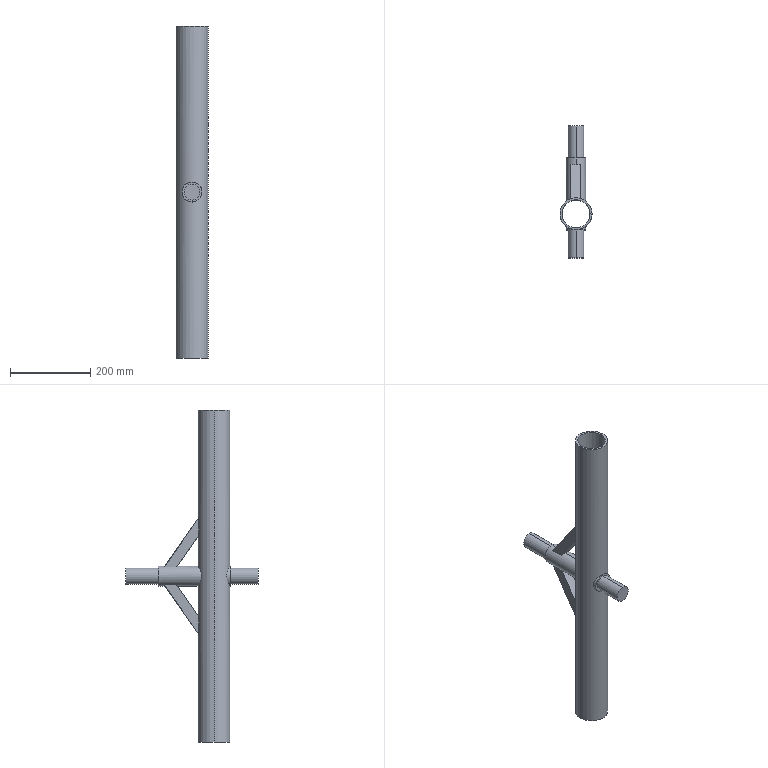Part | SolidWorks | 1 solid | 26 faces | box 80 x 330 x 830 mm | volume 1520421 mm3 | plane 14 | cylinder 12 | commonest cylinder face diameters 40 x4 50 x4 70 x2 80 x2
STEP:
#1=CARTESIAN_POINT('',(0.,140.,20.));
#2=VERTEX_POINT('',#1);
#3=CARTESIAN_POINT('',(0.,140.,-20.));
#4=VERTEX_POINT('',#3);
#5=CARTESIAN_POINT('',(0.,140.,0.));
#6=DIRECTION('',(0.,1.,0.));
#7=DIRECTION('',(0.,0.,1.));
#8=AXIS2_PLACEMENT_3D('',#5,#6,#7);
#9=CIRCLE('',#8,20.);
#10=EDGE_CURVE('',#2,#4,#9,.T.);
#11=ORIENTED_EDGE('',*,*,#10,.T.);
#12=CARTESIAN_POINT('',(0.,220.,-20.));
#13=VERTEX_POINT('',#12);
#14=CARTESIAN_POINT('',(0.,-236.569,-20.));
#15=DIRECTION('',(0.,1.,0.));
#16=VECTOR('',#15,1000.);
#17=LINE('',#14,#16);
#18=EDGE_CURVE('',#4,#13,#17,.T.);
#19=ORIENTED_EDGE('',*,*,#18,.T.);
#20=CARTESIAN_POINT('',(0.,220.,20.));
#21=VERTEX_POINT('',#20);
#22=CARTESIAN_POINT('',(0.,220.,0.));
#23=DIRECTION('',(0.,1.,0.));
#24=DIRECTION('',(0.,0.,1.));
#25=AXIS2_PLACEMENT_3D('',#22,#23,#24);
#26=CIRCLE('',#25,20.);
#27=EDGE_CURVE('',#21,#13,#26,.T.);
#28=ORIENTED_EDGE('',*,*,#27,.F.);
#29=CARTESIAN_POINT('',(0.,-236.569,20.));
#30=DIRECTION('',(0.,1.,0.));
#31=VECTOR('',#30,1000.);
#32=LINE('',#29,#31);
#33=EDGE_CURVE('',#2,#21,#32,.T.);
#34=ORIENTED_EDGE('',*,*,#33,.F.);
#35=EDGE_LOOP('',(#11,#19,#28,#34));
#36=FACE_OUTER_BOUND('',#35,.T.);
#37=CARTESIAN_POINT('',(0.,-236.569,0.));
#38=DIRECTION('',(0.,1.,0.));
#39=DIRECTION('',(0.,0.,1.));
#40=AXIS2_PLACEMENT_3D('',#37,#38,#39);
#41=CYLINDRICAL_SURFACE('',#40,20.);
#42=ADVANCED_FACE('',(#36),#41,.T.);
#43=CARTESIAN_POINT('',(0.,-110.,-20.));
#44=VERTEX_POINT('',#43);
#45=CARTESIAN_POINT('',(0.,-110.,20.));
#46=VERTEX_POINT('',#45);
#47=CARTESIAN_POINT('',(0.,-110.,0.));
#48=DIRECTION('',(0.,-1.,0.));
#49=DIRECTION('',(0.,0.,1.));
#50=AXIS2_PLACEMENT_3D('',#47,#48,#49);
#51=CIRCLE('',#50,20.);
#52=EDGE_CURVE('',#44,#46,#51,.T.);
#53=ORIENTED_EDGE('',*,*,#52,.F.);
#54=CARTESIAN_POINT('',(0.,-40.,-20.));
#55=VERTEX_POINT('',#54);
#56=CARTESIAN_POINT('',(0.,-236.569,-20.));
#57=DIRECTION('',(0.,1.,0.));
#58=VECTOR('',#57,1000.);
#59=LINE('',#56,#58);
#60=EDGE_CURVE('',#44,#55,#59,.T.);
#61=ORIENTED_EDGE('',*,*,#60,.T.);
#62=CARTESIAN_POINT('',(0.,-40.,20.));
#63=VERTEX_POINT('',#62);
#64=CARTESIAN_POINT('',(0.,-40.,0.));
#65=DIRECTION('',(0.,1.,0.));
#66=DIRECTION('',(0.,0.,1.));
#67=AXIS2_PLACEMENT_3D('',#64,#65,#66);
#68=CIRCLE('',#67,20.);
#69=EDGE_CURVE('',#63,#55,#68,.T.);
#70=ORIENTED_EDGE('',*,*,#69,.F.);
#71=CARTESIAN_POINT('',(0.,-236.569,20.));
#72=DIRECTION('',(0.,1.,0.));
#73=VECTOR('',#72,1000.);
#74=LINE('',#71,#73);
#75=EDGE_CURVE('',#46,#63,#74,.T.);
#76=ORIENTED_EDGE('',*,*,#75,.F.);
#77=EDGE_LOOP('',(#53,#61,#70,#76));
#78=FACE_OUTER_BOUND('',#77,.T.);
#79=CARTESIAN_POINT('',(0.,-236.569,0.));
#80=DIRECTION('',(0.,1.,0.));
#81=DIRECTION('',(0.,0.,1.));
#82=AXIS2_PLACEMENT_3D('',#79,#80,#81);
#83=CYLINDRICAL_SURFACE('',#82,20.);
#84=ADVANCED_FACE('',(#78),#83,.T.);
#85=CARTESIAN_POINT('',(0.,40.,-25.));
#86=VERTEX_POINT('',#85);
#87=CARTESIAN_POINT('',(0.,40.,25.));
#88=VERTEX_POINT('',#87);
#89=CARTESIAN_POINT('',(0.,40.,-25.));
#90=CARTESIAN_POINT('',(1.686,40.,-25.));
#91=CARTESIAN_POINT('',(3.35,39.894,-24.831));
#92=CARTESIAN_POINT('',(5.812,39.584,-24.329));
#93=CARTESIAN_POINT('',(6.63,39.455,-24.119));
#94=CARTESIAN_POINT('',(8.216,39.155,-23.626));
#95=CARTESIAN_POINT('',(8.989,38.985,-23.342));
#96=CARTESIAN_POINT('',(10.497,38.606,-22.704));
#97=CARTESIAN_POINT('',(11.232,38.398,-22.35));
#98=CARTESIAN_POINT('',(12.307,38.062,-21.765));
#99=CARTESIAN_POINT('',(12.661,37.945,-21.561));
#100=CARTESIAN_POINT('',(13.355,37.706,-21.138));
#101=CARTESIAN_POINT('',(13.695,37.584,-20.919));
#102=CARTESIAN_POINT('',(15.361,36.96,-19.789));
#103=CARTESIAN_POINT('',(16.586,36.421,-18.773));
#104=CARTESIAN_POINT('',(18.275,35.587,-17.078));
#105=CARTESIAN_POINT('',(18.814,35.304,-16.483));
#106=CARTESIAN_POINT('',(19.824,34.747,-15.253));
#107=CARTESIAN_POINT('',(20.297,34.472,-14.617));
#108=CARTESIAN_POINT('',(21.626,33.666,-12.642));
#109=CARTESIAN_POINT('',(22.391,33.155,-11.239));
#110=CARTESIAN_POINT('',(23.348,32.481,-8.975));
#111=CARTESIAN_POINT('',(23.63,32.276,-8.204));
#112=CARTESIAN_POINT('',(24.117,31.913,-6.636));
#113=CARTESIAN_POINT('',(24.323,31.756,-5.838));
#114=CARTESIAN_POINT('',(24.574,31.562,-4.617));
#115=CARTESIAN_POINT('',(24.647,31.504,-4.206));
#116=CARTESIAN_POINT('',(24.775,31.404,-3.376));
#117=CARTESIAN_POINT('',(24.828,31.362,-2.956));
#118=CARTESIAN_POINT('',(24.957,31.26,-1.692));
#119=CARTESIAN_POINT('',(25.,31.225,-0.8513));
#120=CARTESIAN_POINT('',(25.,31.225,0.8251));
#121=CARTESIAN_POINT('',(24.959,31.258,1.661));
#122=CARTESIAN_POINT('',(24.833,31.358,2.911));
#123=CARTESIAN_POINT('',(24.781,31.399,3.328));
#124=CARTESIAN_POINT('',(24.655,31.498,4.159));
#125=CARTESIAN_POINT('',(24.581,31.556,4.575));
#126=CARTESIAN_POINT('',(24.163,31.88,6.629));
#127=CARTESIAN_POINT('',(23.675,32.251,8.196));
#128=CARTESIAN_POINT('',(22.725,32.92,10.452));
#129=CARTESIAN_POINT('',(22.371,33.163,11.189));
#130=CARTESIAN_POINT('',(21.604,33.667,12.607));
#131=CARTESIAN_POINT('',(21.189,33.931,13.291));
#132=CARTESIAN_POINT('',(20.3,34.47,14.614));
#133=CARTESIAN_POINT('',(19.824,34.747,15.253));
#134=CARTESIAN_POINT('',(18.811,35.306,16.486));
#135=CARTESIAN_POINT('',(18.271,35.589,17.082));
#136=CARTESIAN_POINT('',(16.585,36.421,18.774));
#137=CARTESIAN_POINT('',(15.363,36.959,19.788));
#138=CARTESIAN_POINT('',(13.372,37.705,21.139));
#139=CARTESIAN_POINT('',(12.681,37.944,21.561));
#140=CARTESIAN_POINT('',(11.242,38.395,22.345));
#141=CARTESIAN_POINT('',(10.504,38.604,22.701));
#142=CARTESIAN_POINT('',(8.248,39.171,23.657));
#143=CARTESIAN_POINT('',(6.682,39.472,24.148));
#144=CARTESIAN_POINT('',(4.638,39.732,24.57));
#145=CARTESIAN_POINT('',(4.224,39.779,24.644));
#146=CARTESIAN_POINT('',(3.389,39.858,24.773));
#147=CARTESIAN_POINT('',(2.967,39.892,24.827));
#148=CARTESIAN_POINT('',(2.123,39.946,24.913));
#149=CARTESIAN_POINT('',(1.7,39.966,24.946));
#150=CARTESIAN_POINT('',(0.8513,39.993,24.989));
#151=CARTESIAN_POINT('',(0.4246,40.,25.));
#152=CARTESIAN_POINT('',(0.,40.,25.));
#153=B_SPLINE_CURVE_WITH_KNOTS('',3,(#89,#90,#91,#92,#93,#94,#95,#96,#97,#98,#99,#100,#101,#102,#103,#104,#105,#106,#107,#108,#109,#110,#111,#112,#113,#114,#115,#116,#117,#118,#119,#120,#121,#122,#123,#124,#125,#126,#127,#128,#129,#130,#131,#132,#133,#134,#135,#136,#137,#138,#139,#140,#141,#142,#143,#144,#145,#146,#147,#148,#149,#150,#151,#152),.UNSPECIFIED.,.F.,.F.,(4,2,2,2,2,2,2,2,2,2,2,2,2,2,2,2,2,2,2,2,2,2,2,2,2,2,2,2,2,2,2,4),(0.08042,0.08543,0.08794,0.09045,0.09296,0.09421,0.09546,0.1005,0.103,0.1055,0.1105,0.113,0.1155,0.1168,0.118,0.1205,0.123,0.1243,0.1256,0.1306,0.1331,0.1356,0.1381,0.1406,0.1456,0.1481,0.1506,0.1556,0.1569,0.1582,0.1594,0.1607),.UNSPECIFIED.);
#154=EDGE_CURVE('',#86,#88,#153,.T.);
#155=ORIENTED_EDGE('',*,*,#154,.F.);
#156=CARTESIAN_POINT('',(0.,91.984,-25.));
#157=VERTEX_POINT('',#156);
#158=CARTESIAN_POINT('',(0.,-40.,-25.));
#159=DIRECTION('',(0.,1.,0.));
#160=VECTOR('',#159,1000.);
#161=LINE('',#158,#160);
#162=EDGE_CURVE('',#86,#157,#161,.T.);
#163=ORIENTED_EDGE('',*,*,#162,.T.);
#164=CARTESIAN_POINT('',(12.5,94.328,-21.651));
#165=VERTEX_POINT('',#164);
#166=CARTESIAN_POINT('',(12.5,94.328,-21.651));
#167=CARTESIAN_POINT('',(8.677,92.783,-23.858));
#168=CARTESIAN_POINT('',(4.414,91.984,-25.));
#169=CARTESIAN_POINT('',(0.,91.984,-25.));
#170=(BOUNDED_CURVE()B_SPLINE_CURVE(3,(#166,#167,#168,#169),.UNSPECIFIED.,.F.,.T.)B_SPLINE_CURVE_WITH_KNOTS((4,4),(2.618,3.142),.UNSPECIFIED.)CURVE()GEOMETRIC_REPRESENTATION_ITEM()RATIONAL_B_SPLINE_CURVE((1.,0.9773,0.9773,1.))REPRESENTATION_ITEM(''));
#171=EDGE_CURVE('',#165,#157,#170,.T.);
#172=ORIENTED_EDGE('',*,*,#171,.F.);
#173=CARTESIAN_POINT('',(12.5,124.845,-21.651));
#174=VERTEX_POINT('',#173);
#175=CARTESIAN_POINT('',(12.5,-40.,-21.651));
#176=DIRECTION('',(0.,1.,0.));
#177=VECTOR('',#176,1000.);
#178=LINE('',#175,#177);
#179=EDGE_CURVE('',#165,#174,#178,.T.);
#180=ORIENTED_EDGE('',*,*,#179,.T.);
#181=CARTESIAN_POINT('',(0.,122.5,-25.));
#182=VERTEX_POINT('',#181);
#183=CARTESIAN_POINT('',(12.5,124.845,-21.651));
#184=CARTESIAN_POINT('',(8.677,123.3,-23.858));
#185=CARTESIAN_POINT('',(4.414,122.5,-25.));
#186=CARTESIAN_POINT('',(0.,122.5,-25.));
#187=(BOUNDED_CURVE()B_SPLINE_CURVE(3,(#183,#184,#185,#186),.UNSPECIFIED.,.F.,.F.)B_SPLINE_CURVE_WITH_KNOTS((4,4),(2.618,3.142),.UNSPECIFIED.)CURVE()GEOMETRIC_REPRESENTATION_ITEM()RATIONAL_B_SPLINE_CURVE((1.,0.9773,0.9773,1.))REPRESENTATION_ITEM(''));
#188=EDGE_CURVE('',#174,#182,#187,.T.);
#189=ORIENTED_EDGE('',*,*,#188,.T.);
#190=CARTESIAN_POINT('',(0.,140.,-25.));
#191=VERTEX_POINT('',#190);
#192=CARTESIAN_POINT('',(0.,-40.,-25.));
#193=DIRECTION('',(0.,1.,0.));
#194=VECTOR('',#193,1000.);
#195=LINE('',#192,#194);
#196=EDGE_CURVE('',#182,#191,#195,.T.);
#197=ORIENTED_EDGE('',*,*,#196,.T.);
#198=CARTESIAN_POINT('',(0.,140.,25.));
#199=VERTEX_POINT('',#198);
#200=CARTESIAN_POINT('',(0.,140.,0.));
#201=DIRECTION('',(0.,1.,0.));
#202=DIRECTION('',(1.,0.,0.));
#203=AXIS2_PLACEMENT_3D('',#200,#201,#202);
#204=CIRCLE('',#203,25.);
#205=EDGE_CURVE('',#199,#191,#204,.T.);
#206=ORIENTED_EDGE('',*,*,#205,.F.);
#207=CARTESIAN_POINT('',(0.,122.5,25.));
#208=VERTEX_POINT('',#207);
#209=CARTESIAN_POINT('',(0.,-40.,25.));
#210=DIRECTION('',(0.,1.,0.));
#211=VECTOR('',#210,1000.);
#212=LINE('',#209,#211);
#213=EDGE_CURVE('',#208,#199,#212,.T.);
#214=ORIENTED_EDGE('',*,*,#213,.F.);
#215=CARTESIAN_POINT('',(12.5,124.845,21.651));
#216=VERTEX_POINT('',#215);
#217=CARTESIAN_POINT('',(0.,122.5,25.));
#218=CARTESIAN_POINT('',(4.414,122.5,25.));
#219=CARTESIAN_POINT('',(8.677,123.3,23.858));
#220=CARTESIAN_POINT('',(12.5,124.845,21.651));
#221=(BOUNDED_CURVE()B_SPLINE_CURVE(3,(#217,#218,#219,#220),.UNSPECIFIED.,.F.,.F.)B_SPLINE_CURVE_WITH_KNOTS((4,4),(3.142,3.665),.UNSPECIFIED.)CURVE()GEOMETRIC_REPRESENTATION_ITEM()RATIONAL_B_SPLINE_CURVE((1.,0.9773,0.9773,1.))REPRESENTATION_ITEM(''));
#222=EDGE_CURVE('',#208,#216,#221,.T.);
#223=ORIENTED_EDGE('',*,*,#222,.T.);
#224=CARTESIAN_POINT('',(12.5,94.328,21.651));
#225=VERTEX_POINT('',#224);
#226=CARTESIAN_POINT('',(12.5,-40.,21.651));
#227=DIRECTION('',(0.,-1.,0.));
#228=VECTOR('',#227,1000.);
#229=LINE('',#226,#228);
#230=EDGE_CURVE('',#216,#225,#229,.T.);
#231=ORIENTED_EDGE('',*,*,#230,.T.);
#232=CARTESIAN_POINT('',(0.,91.984,25.));
#233=VERTEX_POINT('',#232);
#234=CARTESIAN_POINT('',(0.,91.984,25.));
#235=CARTESIAN_POINT('',(4.414,91.984,25.));
#236=CARTESIAN_POINT('',(8.677,92.783,23.858));
#237=CARTESIAN_POINT('',(12.5,94.328,21.651));
#238=(BOUNDED_CURVE()B_SPLINE_CURVE(3,(#234,#235,#236,#237),.UNSPECIFIED.,.F.,.F.)B_SPLINE_CURVE_WITH_KNOTS((4,4),(3.142,3.665),.UNSPECIFIED.)CURVE()GEOMETRIC_REPRESENTATION_ITEM()RATIONAL_B_SPLINE_CURVE((1.,0.9773,0.9773,1.))REPRESENTATION_ITEM(''));
#239=EDGE_CURVE('',#233,#225,#238,.T.);
#240=ORIENTED_EDGE('',*,*,#239,.F.);
#241=CARTESIAN_POINT('',(0.,-40.,25.));
#242=DIRECTION('',(0.,1.,0.));
#243=VECTOR('',#242,1000.);
#244=LINE('',#241,#243);
#245=EDGE_CURVE('',#88,#233,#244,.T.);
#246=ORIENTED_EDGE('',*,*,#245,.F.);
#247=EDGE_LOOP('',(#155,#163,#172,#180,#189,#197,#206,#214,#223,#231,#240,#246));
#248=FACE_OUTER_BOUND('',#247,.T.);
#249=CARTESIAN_POINT('',(0.,-40.,0.));
#250=DIRECTION('',(0.,1.,0.));
#251=DIRECTION('',(0.,0.,1.));
#252=AXIS2_PLACEMENT_3D('',#249,#250,#251);
#253=CYLINDRICAL_SURFACE('',#252,25.);
#254=ADVANCED_FACE('',(#248),#253,.T.);
#255=CARTESIAN_POINT('',(-35.,0.,415.));
#256=VERTEX_POINT('',#255);
#257=CARTESIAN_POINT('',(35.,0.,415.));
#258=VERTEX_POINT('',#257);
#259=CARTESIAN_POINT('',(0.,0.,415.));
#260=DIRECTION('',(0.,0.,1.));
#261=DIRECTION('',(1.,0.,0.));
#262=AXIS2_PLACEMENT_3D('',#259,#260,#261);
#263=CIRCLE('',#262,35.);
#264=EDGE_CURVE('',#256,#258,#263,.T.);
#265=ORIENTED_EDGE('',*,*,#264,.T.);
#266=CARTESIAN_POINT('',(35.,0.,-415.));
#267=VERTEX_POINT('',#266);
#268=CARTESIAN_POINT('',(35.,0.,415.));
#269=DIRECTION('',(0.,0.,-1.));
#270=VECTOR('',#269,1000.);
#271=LINE('',#268,#270);
#272=EDGE_CURVE('',#258,#267,#271,.T.);
#273=ORIENTED_EDGE('',*,*,#272,.T.);
#274=CARTESIAN_POINT('',(-35.,0.,-415.));
#275=VERTEX_POINT('',#274);
#276=CARTESIAN_POINT('',(0.,0.,-415.));
#277=DIRECTION('',(0.,0.,1.));
#278=DIRECTION('',(1.,0.,0.));
#279=AXIS2_PLACEMENT_3D('',#276,#277,#278);
#280=CIRCLE('',#279,35.);
#281=EDGE_CURVE('',#275,#267,#280,.T.);
#282=ORIENTED_EDGE('',*,*,#281,.F.);
#283=CARTESIAN_POINT('',(-35.,0.,415.));
#284=DIRECTION('',(0.,0.,-1.));
#285=VECTOR('',#284,1000.);
#286=LINE('',#283,#285);
#287=EDGE_CURVE('',#256,#275,#286,.T.);
#288=ORIENTED_EDGE('',*,*,#287,.F.);
#289=EDGE_LOOP('',(#265,#273,#282,#288));
#290=FACE_OUTER_BOUND('',#289,.T.);
#291=CARTESIAN_POINT('',(0.,0.,415.));
#292=DIRECTION('',(0.,0.,-1.));
#293=DIRECTION('',(-1.,0.,0.));
#294=AXIS2_PLACEMENT_3D('',#291,#292,#293);
#295=CYLINDRICAL_SURFACE('',#294,35.);
#296=ADVANCED_FACE('',(#290),#295,.F.);
#297=CARTESIAN_POINT('',(12.5,37.997,-102.124));
#298=VERTEX_POINT('',#297);
#299=CARTESIAN_POINT('',(12.5,37.997,-145.719));
#300=VERTEX_POINT('',#299);
#301=CARTESIAN_POINT('',(12.5,37.997,415.));
#302=DIRECTION('',(0.,0.,-1.));
#303=VECTOR('',#302,1000.);
#304=LINE('',#301,#303);
#305=EDGE_CURVE('',#298,#300,#304,.T.);
#306=ORIENTED_EDGE('',*,*,#305,.F.);
#307=CARTESIAN_POINT('',(-12.5,37.997,-102.124));
#308=VERTEX_POINT('',#307);
#309=CARTESIAN_POINT('',(12.5,37.997,-102.124));
#310=CARTESIAN_POINT('',(4.311,40.691,-98.275));
#311=CARTESIAN_POINT('',(-4.311,40.691,-98.275));
#312=CARTESIAN_POINT('',(-12.5,37.997,-102.124));
#313=(BOUNDED_CURVE()B_SPLINE_CURVE(3,(#309,#310,#311,#312),.UNSPECIFIED.,.F.,.F.)B_SPLINE_CURVE_WITH_KNOTS((4,4),(2.824,3.459),.UNSPECIFIED.)CURVE()GEOMETRIC_REPRESENTATION_ITEM()RATIONAL_B_SPLINE_CURVE((1.,0.9666,0.9666,1.))REPRESENTATION_ITEM(''));
#314=EDGE_CURVE('',#298,#308,#313,.T.);
#315=ORIENTED_EDGE('',*,*,#314,.T.);
#316=CARTESIAN_POINT('',(-12.5,37.997,-145.719));
#317=VERTEX_POINT('',#316);
#318=CARTESIAN_POINT('',(-12.5,37.997,415.));
#319=DIRECTION('',(0.,0.,-1.));
#320=VECTOR('',#319,1000.);
#321=LINE('',#318,#320);
#322=EDGE_CURVE('',#308,#317,#321,.T.);
#323=ORIENTED_EDGE('',*,*,#322,.T.);
#324=CARTESIAN_POINT('',(12.5,37.997,-145.719));
#325=CARTESIAN_POINT('',(4.311,40.691,-141.87));
#326=CARTESIAN_POINT('',(-4.311,40.691,-141.87));
#327=CARTESIAN_POINT('',(-12.5,37.997,-145.719));
#328=(BOUNDED_CURVE()B_SPLINE_CURVE(3,(#324,#325,#326,#327),.UNSPECIFIED.,.F.,.T.)B_SPLINE_CURVE_WITH_KNOTS((4,4),(2.824,3.459),.UNSPECIFIED.)CURVE()GEOMETRIC_REPRESENTATION_ITEM()RATIONAL_B_SPLINE_CURVE((1.,0.9666,0.9666,1.))REPRESENTATION_ITEM(''));
#329=EDGE_CURVE('',#300,#317,#328,.T.);
#330=ORIENTED_EDGE('',*,*,#329,.F.);
#331=EDGE_LOOP('',(#306,#315,#323,#330));
#332=FACE_BOUND('',#331,.T.);
#333=CARTESIAN_POINT('',(0.,40.,25.));
#334=CARTESIAN_POINT('',(-1.702,40.,25.));
#335=CARTESIAN_POINT('',(-3.368,39.892,24.828));
#336=CARTESIAN_POINT('',(-5.816,39.583,24.328));
#337=CARTESIAN_POINT('',(-6.623,39.456,24.121));
#338=CARTESIAN_POINT('',(-8.221,39.154,23.624));
#339=CARTESIAN_POINT('',(-8.998,38.983,23.339));
#340=CARTESIAN_POINT('',(-11.261,38.414,22.38));
#341=CARTESIAN_POINT('',(-12.683,37.963,21.605));
#342=CARTESIAN_POINT('',(-15.369,36.957,19.785));
#343=CARTESIAN_POINT('',(-16.595,36.417,18.765));
#344=CARTESIAN_POINT('',(-18.275,35.587,17.078));
#345=CARTESIAN_POINT('',(-18.808,35.307,16.489));
#346=CARTESIAN_POINT('',(-19.569,34.888,15.564));
#347=CARTESIAN_POINT('',(-19.816,34.748,15.247));
#348=CARTESIAN_POINT('',(-20.294,34.471,14.606));
#349=CARTESIAN_POINT('',(-20.524,34.334,14.28));
#350=CARTESIAN_POINT('',(-21.635,33.66,12.627));
#351=CARTESIAN_POINT('',(-22.396,33.152,11.227));
#352=CARTESIAN_POINT('',(-23.341,32.486,8.991));
#353=CARTESIAN_POINT('',(-23.624,32.28,8.222));
#354=CARTESIAN_POINT('',(-24.118,31.913,6.636));
#355=CARTESIAN_POINT('',(-24.324,31.755,5.833));
#356=CARTESIAN_POINT('',(-24.658,31.497,4.205));
#357=CARTESIAN_POINT('',(-24.785,31.396,3.381));
#358=CARTESIAN_POINT('',(-24.913,31.295,2.127));
#359=CARTESIAN_POINT('',(-24.945,31.269,1.707));
#360=CARTESIAN_POINT('',(-24.989,31.234,0.8596));
#361=CARTESIAN_POINT('',(-25.,31.225,0.4326));
#362=CARTESIAN_POINT('',(-25.001,31.224,-1.685));
#363=CARTESIAN_POINT('',(-24.831,31.363,-3.35));
#364=CARTESIAN_POINT('',(-24.331,31.75,-5.805));
#365=CARTESIAN_POINT('',(-24.122,31.91,-6.619));
#366=CARTESIAN_POINT('',(-23.633,32.273,-8.195));
#367=CARTESIAN_POINT('',(-23.352,32.478,-8.963));
#368=CARTESIAN_POINT('',(-22.721,32.923,-10.461));
#369=CARTESIAN_POINT('',(-22.37,33.163,-11.191));
#370=CARTESIAN_POINT('',(-21.598,33.671,-12.617));
#371=CARTESIAN_POINT('',(-21.18,33.936,-13.305));
#372=CARTESIAN_POINT('',(-19.842,34.747,-15.292));
#373=CARTESIAN_POINT('',(-18.835,35.311,-16.517));
#374=CARTESIAN_POINT('',(-17.423,36.008,-17.933));
#375=CARTESIAN_POINT('',(-17.132,36.147,-18.211));
#376=CARTESIAN_POINT('',(-16.54,36.422,-18.751));
#377=CARTESIAN_POINT('',(-16.238,36.557,-19.013));
#378=CARTESIAN_POINT('',(-15.315,36.958,-19.776));
#379=CARTESIAN_POINT('',(-14.677,37.217,-20.254));
#380=CARTESIAN_POINT('',(-12.69,37.96,-21.599));
#381=CARTESIAN_POINT('',(-11.27,38.412,-22.377));
#382=CARTESIAN_POINT('',(-8.216,39.179,-23.67));
#383=CARTESIAN_POINT('',(-6.64,39.479,-24.159));
#384=CARTESIAN_POINT('',(-4.203,39.787,-24.658));
#385=CARTESIAN_POINT('',(-3.378,39.866,-24.785));
#386=CARTESIAN_POINT('',(-1.701,39.973,-24.956));
#387=CARTESIAN_POINT('',(-0.845,40.,-25.));
#388=CARTESIAN_POINT('',(0.,40.,-25.));
#389=B_SPLINE_CURVE_WITH_KNOTS('',3,(#333,#334,#335,#336,#337,#338,#339,#340,#341,#342,#343,#344,#345,#346,#347,#348,#349,#350,#351,#352,#353,#354,#355,#356,#357,#358,#359,#360,#361,#362,#363,#364,#365,#366,#367,#368,#369,#370,#371,#372,#373,#374,#375,#376,#377,#378,#379,#380,#381,#382,#383,#384,#385,#386,#387,#388),.UNSPECIFIED.,.F.,.F.,(4,2,2,2,2,2,2,2,2,2,2,2,2,2,2,2,2,2,2,2,2,2,2,2,2,2,2,4),(0.,0.005026,0.007539,0.01005,0.01508,0.02011,0.02262,0.02387,0.02513,0.03016,0.03267,0.03518,0.0377,0.03895,0.04021,0.04524,0.04775,0.05026,0.05278,0.05529,0.06032,0.06157,0.06283,0.06534,0.07037,0.07539,0.07791,0.08042),.UNSPECIFIED.);
#390=EDGE_CURVE('',#88,#86,#389,.T.);
#391=ORIENTED_EDGE('',*,*,#390,.T.);
#392=ORIENTED_EDGE('',*,*,#154,.T.);
#393=EDGE_LOOP('',(#391,#392));
#394=FACE_BOUND('',#393,.T.);
#395=CARTESIAN_POINT('',(-12.5,37.997,145.719));
#396=VERTEX_POINT('',#395);
#397=CARTESIAN_POINT('',(12.5,37.997,145.719));
#398=VERTEX_POINT('',#397);
#399=CARTESIAN_POINT('',(-12.5,37.997,145.719));
#400=CARTESIAN_POINT('',(-4.311,40.691,141.87));
#401=CARTESIAN_POINT('',(4.311,40.691,141.87));
#402=CARTESIAN_POINT('',(12.5,37.997,145.719));
#403=(BOUNDED_CURVE()B_SPLINE_CURVE(3,(#399,#400,#401,#402),.UNSPECIFIED.,.F.,.F.)B_SPLINE_CURVE_WITH_KNOTS((4,4),(5.965,6.601),.UNSPECIFIED.)CURVE()GEOMETRIC_REPRESENTATION_ITEM()RATIONAL_B_SPLINE_CURVE((1.,0.9666,0.9666,1.))REPRESENTATION_ITEM(''));
#404=EDGE_CURVE('',#396,#398,#403,.T.);
#405=ORIENTED_EDGE('',*,*,#404,.F.);
#406=CARTESIAN_POINT('',(-12.5,37.997,102.124));
#407=VERTEX_POINT('',#406);
#408=CARTESIAN_POINT('',(-12.5,37.997,415.));
#409=DIRECTION('',(0.,0.,-1.));
#410=VECTOR('',#409,1000.);
#411=LINE('',#408,#410);
#412=EDGE_CURVE('',#396,#407,#411,.T.);
#413=ORIENTED_EDGE('',*,*,#412,.T.);
#414=CARTESIAN_POINT('',(12.5,37.997,102.124));
#415=VERTEX_POINT('',#414);
#416=CARTESIAN_POINT('',(-12.5,37.997,102.124));
#417=CARTESIAN_POINT('',(-4.311,40.691,98.275));
#418=CARTESIAN_POINT('',(4.311,40.691,98.275));
#419=CARTESIAN_POINT('',(12.5,37.997,102.124));
#420=(BOUNDED_CURVE()B_SPLINE_CURVE(3,(#416,#417,#418,#419),.UNSPECIFIED.,.F.,.T.)B_SPLINE_CURVE_WITH_KNOTS((4,4),(5.965,6.601),.UNSPECIFIED.)CURVE()GEOMETRIC_REPRESENTATION_ITEM()RATIONAL_B_SPLINE_CURVE((1.,0.9666,0.9666,1.))REPRESENTATION_ITEM(''));
#421=EDGE_CURVE('',#407,#415,#420,.T.);
#422=ORIENTED_EDGE('',*,*,#421,.T.);
#423=CARTESIAN_POINT('',(12.5,37.997,415.));
#424=DIRECTION('',(0.,0.,-1.));
#425=VECTOR('',#424,1000.);
#426=LINE('',#423,#425);
#427=EDGE_CURVE('',#398,#415,#426,.T.);
#428=ORIENTED_EDGE('',*,*,#427,.F.);
#429=EDGE_LOOP('',(#405,#413,#422,#428));
#430=FACE_BOUND('',#429,.T.);
#431=CARTESIAN_POINT('',(40.,0.,415.));
#432=VERTEX_POINT('',#431);
#433=CARTESIAN_POINT('',(-40.,0.,415.));
#434=VERTEX_POINT('',#433);
#435=CARTESIAN_POINT('',(0.,0.,415.));
#436=DIRECTION('',(0.,0.,1.));
#437=DIRECTION('',(1.,0.,0.));
#438=AXIS2_PLACEMENT_3D('',#435,#436,#437);
#439=CIRCLE('',#438,40.);
#440=EDGE_CURVE('',#432,#434,#439,.T.);
#441=ORIENTED_EDGE('',*,*,#440,.F.);
#442=CARTESIAN_POINT('',(40.,0.,-415.));
#443=VERTEX_POINT('',#442);
#444=CARTESIAN_POINT('',(40.,0.,415.));
#445=DIRECTION('',(0.,0.,-1.));
#446=VECTOR('',#445,1000.);
#447=LINE('',#444,#446);
#448=EDGE_CURVE('',#432,#443,#447,.T.);
#449=ORIENTED_EDGE('',*,*,#448,.T.);
#450=CARTESIAN_POINT('',(-40.,0.,-415.));
#451=VERTEX_POINT('',#450);
#452=CARTESIAN_POINT('',(0.,0.,-415.));
#453=DIRECTION('',(0.,0.,1.));
#454=DIRECTION('',(1.,0.,0.));
#455=AXIS2_PLACEMENT_3D('',#452,#453,#454);
#456=CIRCLE('',#455,40.);
#457=EDGE_CURVE('',#443,#451,#456,.T.);
#458=ORIENTED_EDGE('',*,*,#457,.T.);
#459=CARTESIAN_POINT('',(-40.,0.,415.));
#460=DIRECTION('',(0.,0.,-1.));
#461=VECTOR('',#460,1000.);
#462=LINE('',#459,#461);
#463=EDGE_CURVE('',#434,#451,#462,.T.);
#464=ORIENTED_EDGE('',*,*,#463,.F.);
#465=EDGE_LOOP('',(#441,#449,#458,#464));
#466=FACE_OUTER_BOUND('',#465,.T.);
#467=CARTESIAN_POINT('',(0.,0.,415.));
#468=DIRECTION('',(0.,0.,-1.));
#469=DIRECTION('',(-1.,0.,0.));
#470=AXIS2_PLACEMENT_3D('',#467,#468,#469);
#471=CYLINDRICAL_SURFACE('',#470,40.);
#472=ADVANCED_FACE('',(#332,#394,#430,#466),#471,.T.);
#473=ORIENTED_EDGE('',*,*,#448,.F.);
#474=CARTESIAN_POINT('',(0.,0.,415.));
#475=DIRECTION('',(0.,0.,1.));
#476=DIRECTION('',(1.,0.,0.));
#477=AXIS2_PLACEMENT_3D('',#474,#475,#476);
#478=CIRCLE('',#477,40.);
#479=EDGE_CURVE('',#434,#432,#478,.T.);
#480=ORIENTED_EDGE('',*,*,#479,.F.);
#481=ORIENTED_EDGE('',*,*,#463,.T.);
#482=CARTESIAN_POINT('',(0.,0.,-415.));
#483=DIRECTION('',(0.,0.,1.));
#484=DIRECTION('',(1.,0.,0.));
#485=AXIS2_PLACEMENT_3D('',#482,#483,#484);
#486=CIRCLE('',#485,40.);
#487=EDGE_CURVE('',#451,#443,#486,.T.);
#488=ORIENTED_EDGE('',*,*,#487,.T.);
#489=EDGE_LOOP('',(#473,#480,#481,#488));
#490=FACE_OUTER_BOUND('',#489,.T.);
#491=CARTESIAN_POINT('',(0.,-40.,-25.));
#492=VERTEX_POINT('',#491);
#493=CARTESIAN_POINT('',(0.,-40.,25.));
#494=VERTEX_POINT('',#493);
#495=CARTESIAN_POINT('',(0.,-40.,-25.));
#496=CARTESIAN_POINT('',(-1.686,-40.,-25.));
#497=CARTESIAN_POINT('',(-3.35,-39.894,-24.831));
#498=CARTESIAN_POINT('',(-5.812,-39.584,-24.329));
#499=CARTESIAN_POINT('',(-6.63,-39.455,-24.119));
#500=CARTESIAN_POINT('',(-8.216,-39.155,-23.626));
#501=CARTESIAN_POINT('',(-8.989,-38.985,-23.342));
#502=CARTESIAN_POINT('',(-10.497,-38.606,-22.704));
#503=CARTESIAN_POINT('',(-11.232,-38.398,-22.35));
#504=CARTESIAN_POINT('',(-12.307,-38.062,-21.765));
#505=CARTESIAN_POINT('',(-12.661,-37.945,-21.561));
#506=CARTESIAN_POINT('',(-13.355,-37.706,-21.138));
#507=CARTESIAN_POINT('',(-13.695,-37.584,-20.919));
#508=CARTESIAN_POINT('',(-15.361,-36.96,-19.789));
#509=CARTESIAN_POINT('',(-16.586,-36.421,-18.773));
#510=CARTESIAN_POINT('',(-18.275,-35.587,-17.078));
#511=CARTESIAN_POINT('',(-18.814,-35.304,-16.483));
#512=CARTESIAN_POINT('',(-19.824,-34.747,-15.253));
#513=CARTESIAN_POINT('',(-20.297,-34.472,-14.617));
#514=CARTESIAN_POINT('',(-21.626,-33.666,-12.642));
#515=CARTESIAN_POINT('',(-22.391,-33.155,-11.239));
#516=CARTESIAN_POINT('',(-23.348,-32.481,-8.975));
#517=CARTESIAN_POINT('',(-23.63,-32.276,-8.204));
#518=CARTESIAN_POINT('',(-24.117,-31.913,-6.636));
#519=CARTESIAN_POINT('',(-24.323,-31.756,-5.838));
#520=CARTESIAN_POINT('',(-24.574,-31.562,-4.617));
#521=CARTESIAN_POINT('',(-24.647,-31.504,-4.206));
#522=CARTESIAN_POINT('',(-24.775,-31.404,-3.376));
#523=CARTESIAN_POINT('',(-24.828,-31.362,-2.956));
#524=CARTESIAN_POINT('',(-24.957,-31.26,-1.692));
#525=CARTESIAN_POINT('',(-25.,-31.225,-0.8513));
#526=CARTESIAN_POINT('',(-25.,-31.225,0.8251));
#527=CARTESIAN_POINT('',(-24.959,-31.258,1.661));
#528=CARTESIAN_POINT('',(-24.833,-31.358,2.911));
#529=CARTESIAN_POINT('',(-24.781,-31.399,3.328));
#530=CARTESIAN_POINT('',(-24.655,-31.498,4.159));
#531=CARTESIAN_POINT('',(-24.581,-31.556,4.575));
#532=CARTESIAN_POINT('',(-24.163,-31.88,6.629));
#533=CARTESIAN_POINT('',(-23.675,-32.251,8.196));
#534=CARTESIAN_POINT('',(-22.725,-32.92,10.452));
#535=CARTESIAN_POINT('',(-22.371,-33.163,11.189));
#536=CARTESIAN_POINT('',(-21.604,-33.667,12.607));
#537=CARTESIAN_POINT('',(-21.189,-33.931,13.291));
#538=CARTESIAN_POINT('',(-20.3,-34.47,14.614));
#539=CARTESIAN_POINT('',(-19.824,-34.747,15.253));
#540=CARTESIAN_POINT('',(-18.811,-35.306,16.486));
#541=CARTESIAN_POINT('',(-18.271,-35.589,17.082));
#542=CARTESIAN_POINT('',(-16.585,-36.421,18.774));
#543=CARTESIAN_POINT('',(-15.363,-36.959,19.788));
#544=CARTESIAN_POINT('',(-13.372,-37.705,21.139));
#545=CARTESIAN_POINT('',(-12.681,-37.944,21.561));
#546=CARTESIAN_POINT('',(-11.242,-38.395,22.345));
#547=CARTESIAN_POINT('',(-10.504,-38.604,22.701));
#548=CARTESIAN_POINT('',(-8.248,-39.171,23.657));
#549=CARTESIAN_POINT('',(-6.682,-39.472,24.148));
#550=CARTESIAN_POINT('',(-4.638,-39.732,24.57));
#551=CARTESIAN_POINT('',(-4.224,-39.779,24.644));
#552=CARTESIAN_POINT('',(-3.389,-39.858,24.773));
#553=CARTESIAN_POINT('',(-2.967,-39.892,24.827));
#554=CARTESIAN_POINT('',(-2.123,-39.946,24.913));
#555=CARTESIAN_POINT('',(-1.7,-39.966,24.946));
#556=CARTESIAN_POINT('',(-0.8513,-39.993,24.989));
#557=CARTESIAN_POINT('',(-0.4246,-40.,25.));
#558=CARTESIAN_POINT('',(0.,-40.,25.));
#559=B_SPLINE_CURVE_WITH_KNOTS('',3,(#495,#496,#497,#498,#499,#500,#501,#502,#503,#504,#505,#506,#507,#508,#509,#510,#511,#512,#513,#514,#515,#516,#517,#518,#519,#520,#521,#522,#523,#524,#525,#526,#527,#528,#529,#530,#531,#532,#533,#534,#535,#536,#537,#538,#539,#540,#541,#542,#543,#544,#545,#546,#547,#548,#549,#550,#551,#552,#553,#554,#555,#556,#557,#558),.UNSPECIFIED.,.F.,.F.,(4,2,2,2,2,2,2,2,2,2,2,2,2,2,2,2,2,2,2,2,2,2,2,2,2,2,2,2,2,2,2,4),(0.08042,0.08543,0.08794,0.09045,0.09296,0.09421,0.09546,0.1005,0.103,0.1055,0.1105,0.113,0.1155,0.1168,0.118,0.1205,0.123,0.1243,0.1256,0.1306,0.1331,0.1356,0.1381,0.1406,0.1456,0.1481,0.1506,0.1556,0.1569,0.1582,0.1594,0.1607),.UNSPECIFIED.);
#560=EDGE_CURVE('',#492,#494,#559,.T.);
#561=ORIENTED_EDGE('',*,*,#560,.T.);
#562=CARTESIAN_POINT('',(0.,-40.,25.));
#563=CARTESIAN_POINT('',(1.702,-40.,25.));
#564=CARTESIAN_POINT('',(3.368,-39.892,24.828));
#565=CARTESIAN_POINT('',(5.816,-39.583,24.328));
#566=CARTESIAN_POINT('',(6.623,-39.456,24.121));
#567=CARTESIAN_POINT('',(8.221,-39.154,23.624));
#568=CARTESIAN_POINT('',(8.998,-38.983,23.339));
#569=CARTESIAN_POINT('',(11.261,-38.414,22.38));
#570=CARTESIAN_POINT('',(12.683,-37.963,21.605));
#571=CARTESIAN_POINT('',(15.369,-36.957,19.785));
#572=CARTESIAN_POINT('',(16.595,-36.417,18.765));
#573=CARTESIAN_POINT('',(18.275,-35.587,17.078));
#574=CARTESIAN_POINT('',(18.808,-35.307,16.489));
#575=CARTESIAN_POINT('',(19.569,-34.888,15.564));
#576=CARTESIAN_POINT('',(19.816,-34.748,15.247));
#577=CARTESIAN_POINT('',(20.294,-34.471,14.606));
#578=CARTESIAN_POINT('',(20.524,-34.334,14.28));
#579=CARTESIAN_POINT('',(21.635,-33.66,12.627));
#580=CARTESIAN_POINT('',(22.396,-33.152,11.227));
#581=CARTESIAN_POINT('',(23.341,-32.486,8.991));
#582=CARTESIAN_POINT('',(23.624,-32.28,8.222));
#583=CARTESIAN_POINT('',(24.118,-31.913,6.636));
#584=CARTESIAN_POINT('',(24.324,-31.755,5.833));
#585=CARTESIAN_POINT('',(24.658,-31.497,4.205));
#586=CARTESIAN_POINT('',(24.785,-31.396,3.381));
#587=CARTESIAN_POINT('',(24.913,-31.295,2.127));
#588=CARTESIAN_POINT('',(24.945,-31.269,1.707));
#589=CARTESIAN_POINT('',(24.989,-31.234,0.8596));
#590=CARTESIAN_POINT('',(25.,-31.225,0.4326));
#591=CARTESIAN_POINT('',(25.001,-31.224,-1.685));
#592=CARTESIAN_POINT('',(24.831,-31.363,-3.35));
#593=CARTESIAN_POINT('',(24.331,-31.75,-5.805));
#594=CARTESIAN_POINT('',(24.122,-31.91,-6.619));
#595=CARTESIAN_POINT('',(23.633,-32.273,-8.195));
#596=CARTESIAN_POINT('',(23.352,-32.478,-8.963));
#597=CARTESIAN_POINT('',(22.721,-32.923,-10.461));
#598=CARTESIAN_POINT('',(22.37,-33.163,-11.191));
#599=CARTESIAN_POINT('',(21.598,-33.671,-12.617));
#600=CARTESIAN_POINT('',(21.18,-33.936,-13.305));
#601=CARTESIAN_POINT('',(19.842,-34.747,-15.292));
#602=CARTESIAN_POINT('',(18.835,-35.311,-16.517));
#603=CARTESIAN_POINT('',(17.423,-36.008,-17.933));
#604=CARTESIAN_POINT('',(17.132,-36.147,-18.211));
#605=CARTESIAN_POINT('',(16.54,-36.422,-18.751));
#606=CARTESIAN_POINT('',(16.238,-36.557,-19.013));
#607=CARTESIAN_POINT('',(15.315,-36.958,-19.776));
#608=CARTESIAN_POINT('',(14.677,-37.217,-20.254));
#609=CARTESIAN_POINT('',(12.69,-37.96,-21.599));
#610=CARTESIAN_POINT('',(11.27,-38.412,-22.377));
#611=CARTESIAN_POINT('',(8.216,-39.179,-23.67));
#612=CARTESIAN_POINT('',(6.64,-39.479,-24.159));
#613=CARTESIAN_POINT('',(4.203,-39.787,-24.658));
#614=CARTESIAN_POINT('',(3.378,-39.866,-24.785));
#615=CARTESIAN_POINT('',(1.701,-39.973,-24.956));
#616=CARTESIAN_POINT('',(0.845,-40.,-25.));
#617=CARTESIAN_POINT('',(0.,-40.,-25.));
#618=B_SPLINE_CURVE_WITH_KNOTS('',3,(#562,#563,#564,#565,#566,#567,#568,#569,#570,#571,#572,#573,#574,#575,#576,#577,#578,#579,#580,#581,#582,#583,#584,#585,#586,#587,#588,#589,#590,#591,#592,#593,#594,#595,#596,#597,#598,#599,#600,#601,#602,#603,#604,#605,#606,#607,#608,#609,#610,#611,#612,#613,#614,#615,#616,#617),.UNSPECIFIED.,.F.,.F.,(4,2,2,2,2,2,2,2,2,2,2,2,2,2,2,2,2,2,2,2,2,2,2,2,2,2,2,4),(0.,0.005026,0.007539,0.01005,0.01508,0.02011,0.02262,0.02387,0.02513,0.03016,0.03267,0.03518,0.0377,0.03895,0.04021,0.04524,0.04775,0.05026,0.05278,0.05529,0.06032,0.06157,0.06283,0.06534,0.07037,0.07539,0.07791,0.08042),.UNSPECIFIED.);
#619=EDGE_CURVE('',#494,#492,#618,.T.);
#620=ORIENTED_EDGE('',*,*,#619,.T.);
#621=EDGE_LOOP('',(#561,#620));
#622=FACE_BOUND('',#621,.T.);
#623=CARTESIAN_POINT('',(0.,0.,415.));
#624=DIRECTION('',(0.,0.,-1.));
#625=DIRECTION('',(-1.,0.,0.));
#626=AXIS2_PLACEMENT_3D('',#623,#624,#625);
#627=CYLINDRICAL_SURFACE('',#626,40.);
#628=ADVANCED_FACE('',(#490,#622),#627,.T.);
#629=ORIENTED_EDGE('',*,*,#272,.F.);
#630=CARTESIAN_POINT('',(0.,0.,415.));
#631=DIRECTION('',(0.,0.,1.));
#632=DIRECTION('',(1.,0.,0.));
#633=AXIS2_PLACEMENT_3D('',#630,#631,#632);
#634=CIRCLE('',#633,35.);
#635=EDGE_CURVE('',#258,#256,#634,.T.);
#636=ORIENTED_EDGE('',*,*,#635,.T.);
#637=ORIENTED_EDGE('',*,*,#287,.T.);
#638=CARTESIAN_POINT('',(0.,0.,-415.));
#639=DIRECTION('',(0.,0.,1.));
#640=DIRECTION('',(1.,0.,0.));
#641=AXIS2_PLACEMENT_3D('',#638,#639,#640);
#642=CIRCLE('',#641,35.);
#643=EDGE_CURVE('',#267,#275,#642,.T.);
#644=ORIENTED_EDGE('',*,*,#643,.F.);
#645=EDGE_LOOP('',(#629,#636,#637,#644));
#646=FACE_OUTER_BOUND('',#645,.T.);
#647=CARTESIAN_POINT('',(0.,0.,415.));
#648=DIRECTION('',(0.,0.,-1.));
#649=DIRECTION('',(-1.,0.,0.));
#650=AXIS2_PLACEMENT_3D('',#647,#648,#649);
#651=CYLINDRICAL_SURFACE('',#650,35.);
#652=ADVANCED_FACE('',(#646),#651,.F.);
#653=ORIENTED_EDGE('',*,*,#162,.F.);
#654=ORIENTED_EDGE('',*,*,#390,.F.);
#655=ORIENTED_EDGE('',*,*,#245,.T.);
#656=CARTESIAN_POINT('',(-12.5,94.328,21.651));
#657=VERTEX_POINT('',#656);
#658=CARTESIAN_POINT('',(-12.5,94.328,21.651));
#659=CARTESIAN_POINT('',(-8.677,92.783,23.858));
#660=CARTESIAN_POINT('',(-4.414,91.984,25.));
#661=CARTESIAN_POINT('',(0.,91.984,25.));
#662=(BOUNDED_CURVE()B_SPLINE_CURVE(3,(#658,#659,#660,#661),.UNSPECIFIED.,.F.,.T.)B_SPLINE_CURVE_WITH_KNOTS((4,4),(2.618,3.142),.UNSPECIFIED.)CURVE()GEOMETRIC_REPRESENTATION_ITEM()RATIONAL_B_SPLINE_CURVE((1.,0.9773,0.9773,1.))REPRESENTATION_ITEM(''));
#663=EDGE_CURVE('',#657,#233,#662,.T.);
#664=ORIENTED_EDGE('',*,*,#663,.F.);
#665=CARTESIAN_POINT('',(-12.5,124.845,21.651));
#666=VERTEX_POINT('',#665);
#667=CARTESIAN_POINT('',(-12.5,-40.,21.651));
#668=DIRECTION('',(0.,-1.,0.));
#669=VECTOR('',#668,1000.);
#670=LINE('',#667,#669);
#671=EDGE_CURVE('',#666,#657,#670,.T.);
#672=ORIENTED_EDGE('',*,*,#671,.F.);
#673=CARTESIAN_POINT('',(-12.5,124.845,21.651));
#674=CARTESIAN_POINT('',(-8.677,123.3,23.858));
#675=CARTESIAN_POINT('',(-4.414,122.5,25.));
#676=CARTESIAN_POINT('',(0.,122.5,25.));
#677=(BOUNDED_CURVE()B_SPLINE_CURVE(3,(#673,#674,#675,#676),.UNSPECIFIED.,.F.,.F.)B_SPLINE_CURVE_WITH_KNOTS((4,4),(2.618,3.142),.UNSPECIFIED.)CURVE()GEOMETRIC_REPRESENTATION_ITEM()RATIONAL_B_SPLINE_CURVE((1.,0.9773,0.9773,1.))REPRESENTATION_ITEM(''));
#678=EDGE_CURVE('',#666,#208,#677,.T.);
#679=ORIENTED_EDGE('',*,*,#678,.T.);
#680=ORIENTED_EDGE('',*,*,#213,.T.);
#681=CARTESIAN_POINT('',(0.,140.,0.));
#682=DIRECTION('',(0.,1.,0.));
#683=DIRECTION('',(1.,0.,0.));
#684=AXIS2_PLACEMENT_3D('',#681,#682,#683);
#685=CIRCLE('',#684,25.);
#686=EDGE_CURVE('',#191,#199,#685,.T.);
#687=ORIENTED_EDGE('',*,*,#686,.F.);
#688=ORIENTED_EDGE('',*,*,#196,.F.);
#689=CARTESIAN_POINT('',(-12.5,124.845,-21.651));
#690=VERTEX_POINT('',#689);
#691=CARTESIAN_POINT('',(0.,122.5,-25.));
#692=CARTESIAN_POINT('',(-4.414,122.5,-25.));
#693=CARTESIAN_POINT('',(-8.677,123.3,-23.858));
#694=CARTESIAN_POINT('',(-12.5,124.845,-21.651));
#695=(BOUNDED_CURVE()B_SPLINE_CURVE(3,(#691,#692,#693,#694),.UNSPECIFIED.,.F.,.F.)B_SPLINE_CURVE_WITH_KNOTS((4,4),(3.142,3.665),.UNSPECIFIED.)CURVE()GEOMETRIC_REPRESENTATION_ITEM()RATIONAL_B_SPLINE_CURVE((1.,0.9773,0.9773,1.))REPRESENTATION_ITEM(''));
#696=EDGE_CURVE('',#182,#690,#695,.T.);
#697=ORIENTED_EDGE('',*,*,#696,.T.);
#698=CARTESIAN_POINT('',(-12.5,94.328,-21.651));
#699=VERTEX_POINT('',#698);
#700=CARTESIAN_POINT('',(-12.5,-40.,-21.651));
#701=DIRECTION('',(0.,1.,0.));
#702=VECTOR('',#701,1000.);
#703=LINE('',#700,#702);
#704=EDGE_CURVE('',#699,#690,#703,.T.);
#705=ORIENTED_EDGE('',*,*,#704,.F.);
#706=CARTESIAN_POINT('',(0.,91.984,-25.));
#707=CARTESIAN_POINT('',(-4.414,91.984,-25.));
#708=CARTESIAN_POINT('',(-8.677,92.783,-23.858));
#709=CARTESIAN_POINT('',(-12.5,94.328,-21.651));
#710=(BOUNDED_CURVE()B_SPLINE_CURVE(3,(#706,#707,#708,#709),.UNSPECIFIED.,.F.,.F.)B_SPLINE_CURVE_WITH_KNOTS((4,4),(3.142,3.665),.UNSPECIFIED.)CURVE()GEOMETRIC_REPRESENTATION_ITEM()RATIONAL_B_SPLINE_CURVE((1.,0.9773,0.9773,1.))REPRESENTATION_ITEM(''));
#711=EDGE_CURVE('',#157,#699,#710,.T.);
#712=ORIENTED_EDGE('',*,*,#711,.F.);
#713=EDGE_LOOP('',(#653,#654,#655,#664,#672,#679,#680,#687,#688,#697,#705,#712));
#714=FACE_OUTER_BOUND('',#713,.T.);
#715=CARTESIAN_POINT('',(0.,-40.,0.));
#716=DIRECTION('',(0.,1.,0.));
#717=DIRECTION('',(0.,0.,1.));
#718=AXIS2_PLACEMENT_3D('',#715,#716,#717);
#719=CYLINDRICAL_SURFACE('',#718,25.);
#720=ADVANCED_FACE('',(#714),#719,.T.);
#721=ORIENTED_EDGE('',*,*,#479,.T.);
#722=ORIENTED_EDGE('',*,*,#440,.T.);
#723=EDGE_LOOP('',(#721,#722));
#724=FACE_OUTER_BOUND('',#723,.T.);
#725=ORIENTED_EDGE('',*,*,#264,.F.);
#726=ORIENTED_EDGE('',*,*,#635,.F.);
#727=EDGE_LOOP('',(#725,#726));
#728=FACE_BOUND('',#727,.T.);
#729=CARTESIAN_POINT('',(0.,0.,415.));
#730=DIRECTION('',(0.,0.,1.));
#731=DIRECTION('',(1.,0.,0.));
#732=AXIS2_PLACEMENT_3D('',#729,#730,#731);
#733=PLANE('',#732);
#734=ADVANCED_FACE('',(#724,#728),#733,.T.);
#735=ORIENTED_EDGE('',*,*,#487,.F.);
#736=ORIENTED_EDGE('',*,*,#457,.F.);
#737=EDGE_LOOP('',(#735,#736));
#738=FACE_OUTER_BOUND('',#737,.T.);
#739=ORIENTED_EDGE('',*,*,#281,.T.);
#740=ORIENTED_EDGE('',*,*,#643,.T.);
#741=EDGE_LOOP('',(#739,#740));
#742=FACE_BOUND('',#741,.T.);
#743=CARTESIAN_POINT('',(0.,0.,-415.));
#744=DIRECTION('',(0.,0.,1.));
#745=DIRECTION('',(1.,0.,0.));
#746=AXIS2_PLACEMENT_3D('',#743,#744,#745);
#747=PLANE('',#746);
#748=ADVANCED_FACE('',(#738,#742),#747,.F.);
#749=ORIENTED_EDGE('',*,*,#205,.T.);
#750=ORIENTED_EDGE('',*,*,#686,.T.);
#751=EDGE_LOOP('',(#749,#750));
#752=FACE_OUTER_BOUND('',#751,.T.);
#753=ORIENTED_EDGE('',*,*,#10,.F.);
#754=CARTESIAN_POINT('',(0.,140.,0.));
#755=DIRECTION('',(0.,1.,0.));
#756=DIRECTION('',(0.,0.,1.));
#757=AXIS2_PLACEMENT_3D('',#754,#755,#756);
#758=CIRCLE('',#757,20.);
#759=EDGE_CURVE('',#4,#2,#758,.T.);
#760=ORIENTED_EDGE('',*,*,#759,.F.);
#761=EDGE_LOOP('',(#753,#760));
#762=FACE_BOUND('',#761,.T.);
#763=CARTESIAN_POINT('',(0.,140.,0.));
#764=DIRECTION('',(0.,1.,0.));
#765=DIRECTION('',(0.,0.,1.));
#766=AXIS2_PLACEMENT_3D('',#763,#764,#765);
#767=PLANE('',#766);
#768=ADVANCED_FACE('',(#752,#762),#767,.T.);
#769=ORIENTED_EDGE('',*,*,#69,.T.);
#770=CARTESIAN_POINT('',(0.,-40.,0.));
#771=DIRECTION('',(0.,1.,0.));
#772=DIRECTION('',(0.,0.,1.));
#773=AXIS2_PLACEMENT_3D('',#770,#771,#772);
#774=CIRCLE('',#773,20.);
#775=EDGE_CURVE('',#55,#63,#774,.T.);
#776=ORIENTED_EDGE('',*,*,#775,.T.);
#777=EDGE_LOOP('',(#769,#776));
#778=FACE_BOUND('',#777,.T.);
#779=CARTESIAN_POINT('',(0.,-40.,0.));
#780=DIRECTION('',(0.,1.,0.));
#781=DIRECTION('',(1.,0.,0.));
#782=AXIS2_PLACEMENT_3D('',#779,#780,#781);
#783=CIRCLE('',#782,25.);
#784=EDGE_CURVE('',#494,#492,#783,.T.);
#785=ORIENTED_EDGE('',*,*,#784,.F.);
#786=CARTESIAN_POINT('',(0.,-40.,0.));
#787=DIRECTION('',(0.,1.,0.));
#788=DIRECTION('',(1.,0.,0.));
#789=AXIS2_PLACEMENT_3D('',#786,#787,#788);
#790=CIRCLE('',#789,25.);
#791=EDGE_CURVE('',#492,#494,#790,.T.);
#792=ORIENTED_EDGE('',*,*,#791,.F.);
#793=EDGE_LOOP('',(#785,#792));
#794=FACE_OUTER_BOUND('',#793,.T.);
#795=CARTESIAN_POINT('',(0.,-40.,0.));
#796=DIRECTION('',(0.,1.,0.));
#797=DIRECTION('',(0.,0.,1.));
#798=AXIS2_PLACEMENT_3D('',#795,#796,#797);
#799=PLANE('',#798);
#800=ADVANCED_FACE('',(#778,#794),#799,.F.);
#801=ORIENTED_EDGE('',*,*,#619,.F.);
#802=ORIENTED_EDGE('',*,*,#784,.T.);
#803=EDGE_LOOP('',(#801,#802));
#804=FACE_OUTER_BOUND('',#803,.T.);
#805=CARTESIAN_POINT('',(0.,-40.,0.));
#806=DIRECTION('',(0.,1.,0.));
#807=DIRECTION('',(0.,0.,1.));
#808=AXIS2_PLACEMENT_3D('',#805,#806,#807);
#809=CYLINDRICAL_SURFACE('',#808,25.);
#810=ADVANCED_FACE('',(#804),#809,.T.);
#811=ORIENTED_EDGE('',*,*,#560,.F.);
#812=ORIENTED_EDGE('',*,*,#791,.T.);
#813=EDGE_LOOP('',(#811,#812));
#814=FACE_OUTER_BOUND('',#813,.T.);
#815=CARTESIAN_POINT('',(0.,-40.,0.));
#816=DIRECTION('',(0.,1.,0.));
#817=DIRECTION('',(0.,0.,1.));
#818=AXIS2_PLACEMENT_3D('',#815,#816,#817);
#819=CYLINDRICAL_SURFACE('',#818,25.);
#820=ADVANCED_FACE('',(#814),#819,.T.);
#821=CARTESIAN_POINT('',(0.,-110.,0.));
#822=DIRECTION('',(0.,-1.,0.));
#823=DIRECTION('',(0.,0.,1.));
#824=AXIS2_PLACEMENT_3D('',#821,#822,#823);
#825=CIRCLE('',#824,20.);
#826=EDGE_CURVE('',#46,#44,#825,.T.);
#827=ORIENTED_EDGE('',*,*,#826,.T.);
#828=ORIENTED_EDGE('',*,*,#52,.T.);
#829=EDGE_LOOP('',(#827,#828));
#830=FACE_OUTER_BOUND('',#829,.T.);
#831=CARTESIAN_POINT('',(0.,-110.,0.));
#832=DIRECTION('',(0.,1.,0.));
#833=DIRECTION('',(0.,0.,1.));
#834=AXIS2_PLACEMENT_3D('',#831,#832,#833);
#835=PLANE('',#834);
#836=ADVANCED_FACE('',(#830),#835,.F.);
#837=ORIENTED_EDGE('',*,*,#60,.F.);
#838=ORIENTED_EDGE('',*,*,#826,.F.);
#839=ORIENTED_EDGE('',*,*,#75,.T.);
#840=ORIENTED_EDGE('',*,*,#775,.F.);
#841=EDGE_LOOP('',(#837,#838,#839,#840));
#842=FACE_OUTER_BOUND('',#841,.T.);
#843=CARTESIAN_POINT('',(0.,-236.569,0.));
#844=DIRECTION('',(0.,1.,0.));
#845=DIRECTION('',(0.,0.,1.));
#846=AXIS2_PLACEMENT_3D('',#843,#844,#845);
#847=CYLINDRICAL_SURFACE('',#846,20.);
#848=ADVANCED_FACE('',(#842),#847,.T.);
#849=ORIENTED_EDGE('',*,*,#18,.F.);
#850=ORIENTED_EDGE('',*,*,#759,.T.);
#851=ORIENTED_EDGE('',*,*,#33,.T.);
#852=CARTESIAN_POINT('',(0.,220.,0.));
#853=DIRECTION('',(0.,1.,0.));
#854=DIRECTION('',(0.,0.,1.));
#855=AXIS2_PLACEMENT_3D('',#852,#853,#854);
#856=CIRCLE('',#855,20.);
#857=EDGE_CURVE('',#13,#21,#856,.T.);
#858=ORIENTED_EDGE('',*,*,#857,.F.);
#859=EDGE_LOOP('',(#849,#850,#851,#858));
#860=FACE_OUTER_BOUND('',#859,.T.);
#861=CARTESIAN_POINT('',(0.,-236.569,0.));
#862=DIRECTION('',(0.,1.,0.));
#863=DIRECTION('',(0.,0.,1.));
#864=AXIS2_PLACEMENT_3D('',#861,#862,#863);
#865=CYLINDRICAL_SURFACE('',#864,20.);
#866=ADVANCED_FACE('',(#860),#865,.T.);
#867=ORIENTED_EDGE('',*,*,#27,.T.);
#868=ORIENTED_EDGE('',*,*,#857,.T.);
#869=EDGE_LOOP('',(#867,#868));
#870=FACE_OUTER_BOUND('',#869,.T.);
#871=CARTESIAN_POINT('',(0.,220.,0.));
#872=DIRECTION('',(0.,1.,0.));
#873=DIRECTION('',(0.,0.,1.));
#874=AXIS2_PLACEMENT_3D('',#871,#872,#873);
#875=PLANE('',#874);
#876=ADVANCED_FACE('',(#870),#875,.T.);
#877=ORIENTED_EDGE('',*,*,#421,.F.);
#878=CARTESIAN_POINT('',(-12.5,119.519,-14.337));
#879=DIRECTION('',(0.,-0.5735,0.8192));
#880=VECTOR('',#879,1000.);
#881=LINE('',#878,#880);
#882=EDGE_CURVE('',#657,#407,#881,.T.);
#883=ORIENTED_EDGE('',*,*,#882,.F.);
#884=ORIENTED_EDGE('',*,*,#663,.T.);
#885=ORIENTED_EDGE('',*,*,#239,.T.);
#886=CARTESIAN_POINT('',(12.5,119.519,-14.337));
#887=DIRECTION('',(0.,-0.5735,0.8192));
#888=VECTOR('',#887,1000.);
#889=LINE('',#886,#888);
#890=EDGE_CURVE('',#225,#415,#889,.T.);
#891=ORIENTED_EDGE('',*,*,#890,.T.);
#892=EDGE_LOOP('',(#877,#883,#884,#885,#891));
#893=FACE_OUTER_BOUND('',#892,.T.);
#894=CARTESIAN_POINT('',(12.5,119.519,-14.337));
#895=DIRECTION('',(0.,-0.8192,-0.5735));
#896=DIRECTION('',(0.,0.5735,-0.8192));
#897=AXIS2_PLACEMENT_3D('',#894,#895,#896);
#898=PLANE('',#897);
#899=ADVANCED_FACE('',(#893),#898,.T.);
#900=CARTESIAN_POINT('',(-12.5,140.,0.));
#901=DIRECTION('',(0.,-0.5735,0.8192));
#902=VECTOR('',#901,1000.);
#903=LINE('',#900,#902);
#904=EDGE_CURVE('',#666,#396,#903,.T.);
#905=ORIENTED_EDGE('',*,*,#904,.T.);
#906=ORIENTED_EDGE('',*,*,#404,.T.);
#907=CARTESIAN_POINT('',(12.5,140.,0.));
#908=DIRECTION('',(0.,-0.5735,0.8192));
#909=VECTOR('',#908,1000.);
#910=LINE('',#907,#909);
#911=EDGE_CURVE('',#216,#398,#910,.T.);
#912=ORIENTED_EDGE('',*,*,#911,.F.);
#913=ORIENTED_EDGE('',*,*,#222,.F.);
#914=ORIENTED_EDGE('',*,*,#678,.F.);
#915=EDGE_LOOP('',(#905,#906,#912,#913,#914));
#916=FACE_OUTER_BOUND('',#915,.T.);
#917=CARTESIAN_POINT('',(12.5,140.,0.));
#918=DIRECTION('',(0.,-0.8192,-0.5735));
#919=DIRECTION('',(0.,0.5735,-0.8192));
#920=AXIS2_PLACEMENT_3D('',#917,#918,#919);
#921=PLANE('',#920);
#922=ADVANCED_FACE('',(#916),#921,.F.);
#923=ORIENTED_EDGE('',*,*,#412,.F.);
#924=ORIENTED_EDGE('',*,*,#904,.F.);
#925=ORIENTED_EDGE('',*,*,#671,.T.);
#926=ORIENTED_EDGE('',*,*,#882,.T.);
#927=EDGE_LOOP('',(#923,#924,#925,#926));
#928=FACE_OUTER_BOUND('',#927,.T.);
#929=CARTESIAN_POINT('',(-12.5,0.,0.));
#930=DIRECTION('',(-1.,0.,0.));
#931=DIRECTION('',(0.,0.,-1.));
#932=AXIS2_PLACEMENT_3D('',#929,#930,#931);
#933=PLANE('',#932);
#934=ADVANCED_FACE('',(#928),#933,.T.);
#935=ORIENTED_EDGE('',*,*,#911,.T.);
#936=ORIENTED_EDGE('',*,*,#427,.T.);
#937=ORIENTED_EDGE('',*,*,#890,.F.);
#938=ORIENTED_EDGE('',*,*,#230,.F.);
#939=EDGE_LOOP('',(#935,#936,#937,#938));
#940=FACE_OUTER_BOUND('',#939,.T.);
#941=CARTESIAN_POINT('',(12.5,0.,0.));
#942=DIRECTION('',(-1.,0.,0.));
#943=DIRECTION('',(0.,0.,-1.));
#944=AXIS2_PLACEMENT_3D('',#941,#942,#943);
#945=PLANE('',#944);
#946=ADVANCED_FACE('',(#940),#945,.F.);
#947=ORIENTED_EDGE('',*,*,#322,.F.);
#948=CARTESIAN_POINT('',(-12.5,119.519,14.337));
#949=DIRECTION('',(0.,-0.5735,-0.8192));
#950=VECTOR('',#949,1000.);
#951=LINE('',#948,#950);
#952=EDGE_CURVE('',#699,#308,#951,.T.);
#953=ORIENTED_EDGE('',*,*,#952,.F.);
#954=ORIENTED_EDGE('',*,*,#704,.T.);
#955=CARTESIAN_POINT('',(-12.5,140.,0.));
#956=DIRECTION('',(0.,-0.5735,-0.8192));
#957=VECTOR('',#956,1000.);
#958=LINE('',#955,#957);
#959=EDGE_CURVE('',#690,#317,#958,.T.);
#960=ORIENTED_EDGE('',*,*,#959,.T.);
#961=EDGE_LOOP('',(#947,#953,#954,#960));
#962=FACE_OUTER_BOUND('',#961,.T.);
#963=CARTESIAN_POINT('',(-12.5,0.,0.));
#964=DIRECTION('',(-1.,0.,0.));
#965=DIRECTION('',(0.,0.,-1.));
#966=AXIS2_PLACEMENT_3D('',#963,#964,#965);
#967=PLANE('',#966);
#968=ADVANCED_FACE('',(#962),#967,.T.);
#969=CARTESIAN_POINT('',(12.5,119.519,14.337));
#970=DIRECTION('',(0.,-0.5735,-0.8192));
#971=VECTOR('',#970,1000.);
#972=LINE('',#969,#971);
#973=EDGE_CURVE('',#165,#298,#972,.T.);
#974=ORIENTED_EDGE('',*,*,#973,.T.);
#975=ORIENTED_EDGE('',*,*,#305,.T.);
#976=CARTESIAN_POINT('',(12.5,140.,0.));
#977=DIRECTION('',(0.,-0.5735,-0.8192));
#978=VECTOR('',#977,1000.);
#979=LINE('',#976,#978);
#980=EDGE_CURVE('',#174,#300,#979,.T.);
#981=ORIENTED_EDGE('',*,*,#980,.F.);
#982=ORIENTED_EDGE('',*,*,#179,.F.);
#983=EDGE_LOOP('',(#974,#975,#981,#982));
#984=FACE_OUTER_BOUND('',#983,.T.);
#985=CARTESIAN_POINT('',(12.5,0.,0.));
#986=DIRECTION('',(-1.,0.,0.));
#987=DIRECTION('',(0.,0.,-1.));
#988=AXIS2_PLACEMENT_3D('',#985,#986,#987);
#989=PLANE('',#988);
#990=ADVANCED_FACE('',(#984),#989,.F.);
#991=ORIENTED_EDGE('',*,*,#314,.F.);
#992=ORIENTED_EDGE('',*,*,#973,.F.);
#993=ORIENTED_EDGE('',*,*,#171,.T.);
#994=ORIENTED_EDGE('',*,*,#711,.T.);
#995=ORIENTED_EDGE('',*,*,#952,.T.);
#996=EDGE_LOOP('',(#991,#992,#993,#994,#995));
#997=FACE_OUTER_BOUND('',#996,.T.);
#998=CARTESIAN_POINT('',(12.5,119.519,14.337));
#999=DIRECTION('',(0.,-0.8192,0.5735));
#1000=DIRECTION('',(0.,0.5735,0.8192));
#1001=AXIS2_PLACEMENT_3D('',#998,#999,#1000);
#1002=PLANE('',#1001);
#1003=ADVANCED_FACE('',(#997),#1002,.T.);
#1004=ORIENTED_EDGE('',*,*,#980,.T.);
#1005=ORIENTED_EDGE('',*,*,#329,.T.);
#1006=ORIENTED_EDGE('',*,*,#959,.F.);
#1007=ORIENTED_EDGE('',*,*,#696,.F.);
#1008=ORIENTED_EDGE('',*,*,#188,.F.);
#1009=EDGE_LOOP('',(#1004,#1005,#1006,#1007,#1008));
#1010=FACE_OUTER_BOUND('',#1009,.T.);
#1011=CARTESIAN_POINT('',(12.5,140.,0.));
#1012=DIRECTION('',(0.,-0.8192,0.5735));
#1013=DIRECTION('',(0.,0.5735,0.8192));
#1014=AXIS2_PLACEMENT_3D('',#1011,#1012,#1013);
#1015=PLANE('',#1014);
#1016=ADVANCED_FACE('',(#1010),#1015,.F.);
#1017=CLOSED_SHELL('',(#42,#84,#254,#296,#472,#628,#652,#720,#734,#748,#768,#800,#810,#820,#836,#848,#866,#876,#899,#922,#934,#946,#968,#990,#1003,#1016));
#1018=MANIFOLD_SOLID_BREP('',#1017);
#1019=CARTESIAN_POINT('',(0.,0.,0.));
#1020=DIRECTION('',(0.,0.,1.));
#1021=DIRECTION('',(1.,0.,0.));
#1022=AXIS2_PLACEMENT_3D('',#1019,#1020,#1021);
#1023=(LENGTH_UNIT()NAMED_UNIT(*)SI_UNIT(.MILLI.,.METRE.));
#1024=UNCERTAINTY_MEASURE_WITH_UNIT(LENGTH_MEASURE(0.00001),#1023,'','');
#1025=(NAMED_UNIT(*)PLANE_ANGLE_UNIT()SI_UNIT($,.RADIAN.));
#1026=(NAMED_UNIT(*)SI_UNIT($,.STERADIAN.)SOLID_ANGLE_UNIT());
#1027=(GEOMETRIC_REPRESENTATION_CONTEXT(3)GLOBAL_UNCERTAINTY_ASSIGNED_CONTEXT((#1024))GLOBAL_UNIT_ASSIGNED_CONTEXT((#1023,#1025,#1026))REPRESENTATION_CONTEXT('',''));
#1028=ADVANCED_BREP_SHAPE_REPRESENTATION('',(#1018,#1022),#1027);